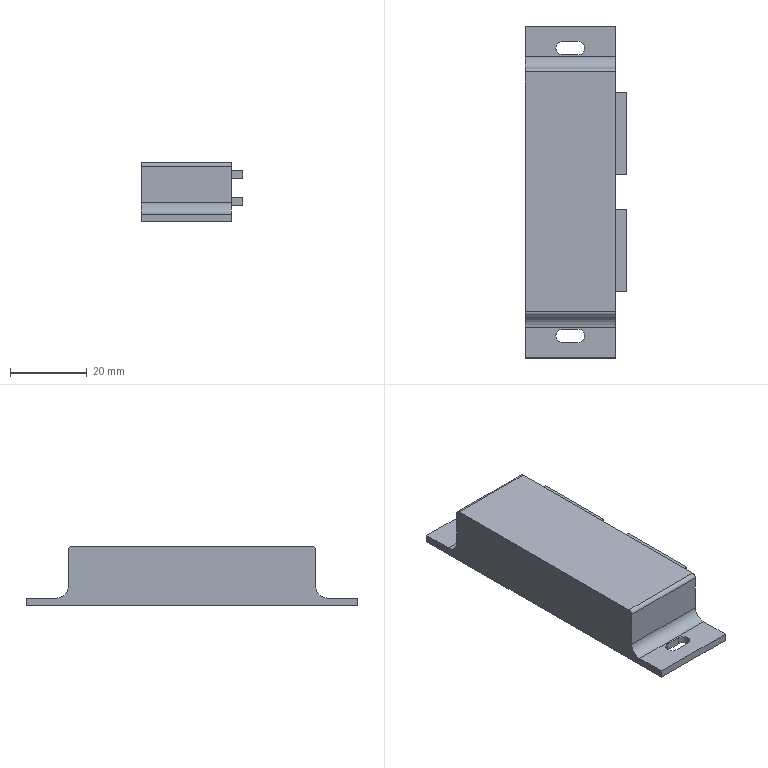Part | SolidWorks | features BaseBody 1 | 1 solid | 44 faces | box 26.5 x 86.5 x 15.5 mm | volume 25030 mm3 | plane 34 | cylinder 10 | commonest cylinder face diameters 3.5 x6 2 x2 6 x2
STEP:
#1=CARTESIAN_POINT('',(-2.,-35.75,2.));
#2=VERTEX_POINT('',#1);
#3=CARTESIAN_POINT('',(-3.75,-37.5,2.));
#4=VERTEX_POINT('',#3);
#5=CARTESIAN_POINT('',(-2.,-37.5,2.));
#6=DIRECTION('',(0.,0.,1.));
#7=DIRECTION('',(-1.,0.,0.));
#8=AXIS2_PLACEMENT_3D('',#5,#6,#7);
#9=CIRCLE('',#8,1.75);
#10=EDGE_CURVE('',#2,#4,#9,.T.);
#11=ORIENTED_EDGE('',*,*,#10,.T.);
#12=CARTESIAN_POINT('',(-3.75,-37.5,0.));
#13=VERTEX_POINT('',#12);
#14=CARTESIAN_POINT('',(-3.75,-37.5,3.));
#15=DIRECTION('',(0.,0.,-1.));
#16=VECTOR('',#15,1000.);
#17=LINE('',#14,#16);
#18=EDGE_CURVE('',#4,#13,#17,.T.);
#19=ORIENTED_EDGE('',*,*,#18,.T.);
#20=CARTESIAN_POINT('',(-2.,-35.75,0.));
#21=VERTEX_POINT('',#20);
#22=CARTESIAN_POINT('',(-2.,-37.5,0.));
#23=DIRECTION('',(0.,0.,1.));
#24=DIRECTION('',(1.,0.,0.));
#25=AXIS2_PLACEMENT_3D('',#22,#23,#24);
#26=CIRCLE('',#25,1.75);
#27=EDGE_CURVE('',#21,#13,#26,.T.);
#28=ORIENTED_EDGE('',*,*,#27,.F.);
#29=CARTESIAN_POINT('',(-2.,-35.75,3.));
#30=DIRECTION('',(0.,0.,-1.));
#31=VECTOR('',#30,1000.);
#32=LINE('',#29,#31);
#33=EDGE_CURVE('',#2,#21,#32,.T.);
#34=ORIENTED_EDGE('',*,*,#33,.F.);
#35=EDGE_LOOP('',(#11,#19,#28,#34));
#36=FACE_OUTER_BOUND('',#35,.T.);
#37=CARTESIAN_POINT('',(-2.,-37.5,3.));
#38=DIRECTION('',(0.,0.,-1.));
#39=DIRECTION('',(-1.,0.,0.));
#40=AXIS2_PLACEMENT_3D('',#37,#38,#39);
#41=CYLINDRICAL_SURFACE('',#40,1.75);
#42=ADVANCED_FACE('',(#36),#41,.F.);
#43=CARTESIAN_POINT('',(-2.,39.25,2.));
#44=VERTEX_POINT('',#43);
#45=CARTESIAN_POINT('',(-3.75,37.5,2.));
#46=VERTEX_POINT('',#45);
#47=CARTESIAN_POINT('',(-2.,37.5,2.));
#48=DIRECTION('',(0.,0.,1.));
#49=DIRECTION('',(-1.,0.,0.));
#50=AXIS2_PLACEMENT_3D('',#47,#48,#49);
#51=CIRCLE('',#50,1.75);
#52=EDGE_CURVE('',#44,#46,#51,.T.);
#53=ORIENTED_EDGE('',*,*,#52,.T.);
#54=CARTESIAN_POINT('',(-3.75,37.5,0.));
#55=VERTEX_POINT('',#54);
#56=CARTESIAN_POINT('',(-3.75,37.5,8.5));
#57=DIRECTION('',(0.,0.,-1.));
#58=VECTOR('',#57,1000.);
#59=LINE('',#56,#58);
#60=EDGE_CURVE('',#46,#55,#59,.T.);
#61=ORIENTED_EDGE('',*,*,#60,.T.);
#62=CARTESIAN_POINT('',(-2.,39.25,0.));
#63=VERTEX_POINT('',#62);
#64=CARTESIAN_POINT('',(-2.,37.5,0.));
#65=DIRECTION('',(0.,0.,-1.));
#66=DIRECTION('',(1.,0.,0.));
#67=AXIS2_PLACEMENT_3D('',#64,#65,#66);
#68=CIRCLE('',#67,1.75);
#69=EDGE_CURVE('',#55,#63,#68,.T.);
#70=ORIENTED_EDGE('',*,*,#69,.T.);
#71=CARTESIAN_POINT('',(-2.,39.25,8.5));
#72=DIRECTION('',(0.,0.,-1.));
#73=VECTOR('',#72,1000.);
#74=LINE('',#71,#73);
#75=EDGE_CURVE('',#44,#63,#74,.T.);
#76=ORIENTED_EDGE('',*,*,#75,.F.);
#77=EDGE_LOOP('',(#53,#61,#70,#76));
#78=FACE_OUTER_BOUND('',#77,.T.);
#79=CARTESIAN_POINT('',(-2.,37.5,8.5));
#80=DIRECTION('',(0.,0.,-1.));
#81=DIRECTION('',(-1.,0.,0.));
#82=AXIS2_PLACEMENT_3D('',#79,#80,#81);
#83=CYLINDRICAL_SURFACE('',#82,1.75);
#84=ADVANCED_FACE('',(#78),#83,.F.);
#85=CARTESIAN_POINT('',(14.75,-4.5,6.3));
#86=VERTEX_POINT('',#85);
#87=CARTESIAN_POINT('',(14.75,-4.5,4.3));
#88=VERTEX_POINT('',#87);
#89=CARTESIAN_POINT('',(14.75,-4.5,15.5));
#90=DIRECTION('',(0.,0.,-1.));
#91=VECTOR('',#90,1000.);
#92=LINE('',#89,#91);
#93=EDGE_CURVE('',#86,#88,#92,.T.);
#94=ORIENTED_EDGE('',*,*,#93,.T.);
#95=CARTESIAN_POINT('',(11.75,-4.5,4.3));
#96=VERTEX_POINT('',#95);
#97=CARTESIAN_POINT('',(14.75,-4.5,4.3));
#98=DIRECTION('',(1.,0.,0.));
#99=VECTOR('',#98,1000.);
#100=LINE('',#97,#99);
#101=EDGE_CURVE('',#96,#88,#100,.T.);
#102=ORIENTED_EDGE('',*,*,#101,.F.);
#103=CARTESIAN_POINT('',(11.75,-4.5,6.3));
#104=VERTEX_POINT('',#103);
#105=CARTESIAN_POINT('',(11.75,-4.5,15.5));
#106=DIRECTION('',(0.,0.,-1.));
#107=VECTOR('',#106,1000.);
#108=LINE('',#105,#107);
#109=EDGE_CURVE('',#104,#96,#108,.T.);
#110=ORIENTED_EDGE('',*,*,#109,.F.);
#111=CARTESIAN_POINT('',(14.75,-4.5,6.3));
#112=DIRECTION('',(-1.,0.,0.));
#113=VECTOR('',#112,1000.);
#114=LINE('',#111,#113);
#115=EDGE_CURVE('',#86,#104,#114,.T.);
#116=ORIENTED_EDGE('',*,*,#115,.F.);
#117=EDGE_LOOP('',(#94,#102,#110,#116));
#118=FACE_OUTER_BOUND('',#117,.T.);
#119=CARTESIAN_POINT('',(11.75,-4.5,15.5));
#120=DIRECTION('',(0.,-1.,0.));
#121=DIRECTION('',(0.,0.,-1.));
#122=AXIS2_PLACEMENT_3D('',#119,#120,#121);
#123=PLANE('',#122);
#124=ADVANCED_FACE('',(#118),#123,.F.);
#125=CARTESIAN_POINT('',(11.75,4.5,4.3));
#126=VERTEX_POINT('',#125);
#127=CARTESIAN_POINT('',(11.75,4.5,6.3));
#128=VERTEX_POINT('',#127);
#129=CARTESIAN_POINT('',(11.75,4.5,0.));
#130=DIRECTION('',(0.,0.,1.));
#131=VECTOR('',#130,1000.);
#132=LINE('',#129,#131);
#133=EDGE_CURVE('',#126,#128,#132,.T.);
#134=ORIENTED_EDGE('',*,*,#133,.F.);
#135=CARTESIAN_POINT('',(14.75,4.5,4.3));
#136=VERTEX_POINT('',#135);
#137=CARTESIAN_POINT('',(14.75,4.5,4.3));
#138=DIRECTION('',(-1.,0.,0.));
#139=VECTOR('',#138,1000.);
#140=LINE('',#137,#139);
#141=EDGE_CURVE('',#136,#126,#140,.T.);
#142=ORIENTED_EDGE('',*,*,#141,.F.);
#143=CARTESIAN_POINT('',(14.75,4.5,6.3));
#144=VERTEX_POINT('',#143);
#145=CARTESIAN_POINT('',(14.75,4.5,0.));
#146=DIRECTION('',(0.,0.,1.));
#147=VECTOR('',#146,1000.);
#148=LINE('',#145,#147);
#149=EDGE_CURVE('',#136,#144,#148,.T.);
#150=ORIENTED_EDGE('',*,*,#149,.T.);
#151=CARTESIAN_POINT('',(14.75,4.5,6.3));
#152=DIRECTION('',(1.,0.,0.));
#153=VECTOR('',#152,1000.);
#154=LINE('',#151,#153);
#155=EDGE_CURVE('',#128,#144,#154,.T.);
#156=ORIENTED_EDGE('',*,*,#155,.F.);
#157=EDGE_LOOP('',(#134,#142,#150,#156));
#158=FACE_OUTER_BOUND('',#157,.T.);
#159=CARTESIAN_POINT('',(11.75,4.5,0.));
#160=DIRECTION('',(0.,1.,0.));
#161=DIRECTION('',(1.,0.,0.));
#162=AXIS2_PLACEMENT_3D('',#159,#160,#161);
#163=PLANE('',#162);
#164=ADVANCED_FACE('',(#158),#163,.F.);
#165=CARTESIAN_POINT('',(11.75,4.5,11.3));
#166=VERTEX_POINT('',#165);
#167=CARTESIAN_POINT('',(11.75,4.5,13.3));
#168=VERTEX_POINT('',#167);
#169=CARTESIAN_POINT('',(11.75,4.5,0.));
#170=DIRECTION('',(0.,0.,1.));
#171=VECTOR('',#170,1000.);
#172=LINE('',#169,#171);
#173=EDGE_CURVE('',#166,#168,#172,.T.);
#174=ORIENTED_EDGE('',*,*,#173,.F.);
#175=CARTESIAN_POINT('',(14.75,4.5,11.3));
#176=VERTEX_POINT('',#175);
#177=CARTESIAN_POINT('',(14.75,4.5,11.3));
#178=DIRECTION('',(-1.,0.,0.));
#179=VECTOR('',#178,1000.);
#180=LINE('',#177,#179);
#181=EDGE_CURVE('',#176,#166,#180,.T.);
#182=ORIENTED_EDGE('',*,*,#181,.F.);
#183=CARTESIAN_POINT('',(14.75,4.5,13.3));
#184=VERTEX_POINT('',#183);
#185=CARTESIAN_POINT('',(14.75,4.5,0.));
#186=DIRECTION('',(0.,0.,1.));
#187=VECTOR('',#186,1000.);
#188=LINE('',#185,#187);
#189=EDGE_CURVE('',#176,#184,#188,.T.);
#190=ORIENTED_EDGE('',*,*,#189,.T.);
#191=CARTESIAN_POINT('',(14.75,4.5,13.3));
#192=DIRECTION('',(1.,0.,0.));
#193=VECTOR('',#192,1000.);
#194=LINE('',#191,#193);
#195=EDGE_CURVE('',#168,#184,#194,.T.);
#196=ORIENTED_EDGE('',*,*,#195,.F.);
#197=EDGE_LOOP('',(#174,#182,#190,#196));
#198=FACE_OUTER_BOUND('',#197,.T.);
#199=CARTESIAN_POINT('',(11.75,4.5,0.));
#200=DIRECTION('',(0.,1.,0.));
#201=DIRECTION('',(1.,0.,0.));
#202=AXIS2_PLACEMENT_3D('',#199,#200,#201);
#203=PLANE('',#202);
#204=ADVANCED_FACE('',(#198),#203,.F.);
#205=CARTESIAN_POINT('',(14.75,-4.5,13.3));
#206=VERTEX_POINT('',#205);
#207=CARTESIAN_POINT('',(14.75,-4.5,11.3));
#208=VERTEX_POINT('',#207);
#209=CARTESIAN_POINT('',(14.75,-4.5,0.));
#210=DIRECTION('',(0.,0.,-1.));
#211=VECTOR('',#210,1000.);
#212=LINE('',#209,#211);
#213=EDGE_CURVE('',#206,#208,#212,.T.);
#214=ORIENTED_EDGE('',*,*,#213,.T.);
#215=CARTESIAN_POINT('',(11.75,-4.5,11.3));
#216=VERTEX_POINT('',#215);
#217=CARTESIAN_POINT('',(14.75,-4.5,11.3));
#218=DIRECTION('',(1.,0.,0.));
#219=VECTOR('',#218,1000.);
#220=LINE('',#217,#219);
#221=EDGE_CURVE('',#216,#208,#220,.T.);
#222=ORIENTED_EDGE('',*,*,#221,.F.);
#223=CARTESIAN_POINT('',(11.75,-4.5,13.3));
#224=VERTEX_POINT('',#223);
#225=CARTESIAN_POINT('',(11.75,-4.5,15.5));
#226=DIRECTION('',(0.,0.,-1.));
#227=VECTOR('',#226,1000.);
#228=LINE('',#225,#227);
#229=EDGE_CURVE('',#224,#216,#228,.T.);
#230=ORIENTED_EDGE('',*,*,#229,.F.);
#231=CARTESIAN_POINT('',(14.75,-4.5,13.3));
#232=DIRECTION('',(-1.,0.,0.));
#233=VECTOR('',#232,1000.);
#234=LINE('',#231,#233);
#235=EDGE_CURVE('',#206,#224,#234,.T.);
#236=ORIENTED_EDGE('',*,*,#235,.F.);
#237=EDGE_LOOP('',(#214,#222,#230,#236));
#238=FACE_OUTER_BOUND('',#237,.T.);
#239=CARTESIAN_POINT('',(11.75,-4.5,15.5));
#240=DIRECTION('',(0.,-1.,0.));
#241=DIRECTION('',(0.,0.,-1.));
#242=AXIS2_PLACEMENT_3D('',#239,#240,#241);
#243=PLANE('',#242);
#244=ADVANCED_FACE('',(#238),#243,.F.);
#245=CARTESIAN_POINT('',(2.,-35.75,2.));
#246=VERTEX_POINT('',#245);
#247=CARTESIAN_POINT('',(11.75,-35.75,2.));
#248=DIRECTION('',(-1.,0.,0.));
#249=VECTOR('',#248,1000.);
#250=LINE('',#247,#249);
#251=EDGE_CURVE('',#246,#2,#250,.T.);
#252=ORIENTED_EDGE('',*,*,#251,.T.);
#253=ORIENTED_EDGE('',*,*,#33,.T.);
#254=CARTESIAN_POINT('',(2.,-35.75,0.));
#255=VERTEX_POINT('',#254);
#256=CARTESIAN_POINT('',(2.,-35.75,0.));
#257=DIRECTION('',(-1.,0.,0.));
#258=VECTOR('',#257,1000.);
#259=LINE('',#256,#258);
#260=EDGE_CURVE('',#255,#21,#259,.T.);
#261=ORIENTED_EDGE('',*,*,#260,.F.);
#262=CARTESIAN_POINT('',(2.,-35.75,3.));
#263=DIRECTION('',(0.,0.,-1.));
#264=VECTOR('',#263,1000.);
#265=LINE('',#262,#264);
#266=EDGE_CURVE('',#246,#255,#265,.T.);
#267=ORIENTED_EDGE('',*,*,#266,.F.);
#268=EDGE_LOOP('',(#252,#253,#261,#267));
#269=FACE_OUTER_BOUND('',#268,.T.);
#270=CARTESIAN_POINT('',(2.,-35.75,3.));
#271=DIRECTION('',(0.,-1.,0.));
#272=DIRECTION('',(0.,0.,-1.));
#273=AXIS2_PLACEMENT_3D('',#270,#271,#272);
#274=PLANE('',#273);
#275=ADVANCED_FACE('',(#269),#274,.T.);
#276=CARTESIAN_POINT('',(2.,-39.25,2.));
#277=VERTEX_POINT('',#276);
#278=CARTESIAN_POINT('',(2.,-37.5,2.));
#279=DIRECTION('',(0.,0.,1.));
#280=DIRECTION('',(-1.,0.,0.));
#281=AXIS2_PLACEMENT_3D('',#278,#279,#280);
#282=CIRCLE('',#281,1.75);
#283=EDGE_CURVE('',#277,#246,#282,.T.);
#284=ORIENTED_EDGE('',*,*,#283,.T.);
#285=ORIENTED_EDGE('',*,*,#266,.T.);
#286=CARTESIAN_POINT('',(2.,-39.25,0.));
#287=VERTEX_POINT('',#286);
#288=CARTESIAN_POINT('',(2.,-37.5,0.));
#289=DIRECTION('',(0.,0.,1.));
#290=DIRECTION('',(1.,0.,0.));
#291=AXIS2_PLACEMENT_3D('',#288,#289,#290);
#292=CIRCLE('',#291,1.75);
#293=EDGE_CURVE('',#287,#255,#292,.T.);
#294=ORIENTED_EDGE('',*,*,#293,.F.);
#295=CARTESIAN_POINT('',(2.,-39.25,3.));
#296=DIRECTION('',(0.,0.,-1.));
#297=VECTOR('',#296,1000.);
#298=LINE('',#295,#297);
#299=EDGE_CURVE('',#277,#287,#298,.T.);
#300=ORIENTED_EDGE('',*,*,#299,.F.);
#301=EDGE_LOOP('',(#284,#285,#294,#300));
#302=FACE_OUTER_BOUND('',#301,.T.);
#303=CARTESIAN_POINT('',(2.,-37.5,3.));
#304=DIRECTION('',(0.,0.,-1.));
#305=DIRECTION('',(-1.,0.,0.));
#306=AXIS2_PLACEMENT_3D('',#303,#304,#305);
#307=CYLINDRICAL_SURFACE('',#306,1.75);
#308=ADVANCED_FACE('',(#302),#307,.F.);
#309=CARTESIAN_POINT('',(-2.,-39.25,2.));
#310=VERTEX_POINT('',#309);
#311=CARTESIAN_POINT('',(11.75,-39.25,2.));
#312=DIRECTION('',(1.,0.,0.));
#313=VECTOR('',#312,1000.);
#314=LINE('',#311,#313);
#315=EDGE_CURVE('',#310,#277,#314,.T.);
#316=ORIENTED_EDGE('',*,*,#315,.T.);
#317=ORIENTED_EDGE('',*,*,#299,.T.);
#318=CARTESIAN_POINT('',(-2.,-39.25,0.));
#319=VERTEX_POINT('',#318);
#320=CARTESIAN_POINT('',(-2.,-39.25,0.));
#321=DIRECTION('',(1.,0.,0.));
#322=VECTOR('',#321,1000.);
#323=LINE('',#320,#322);
#324=EDGE_CURVE('',#319,#287,#323,.T.);
#325=ORIENTED_EDGE('',*,*,#324,.F.);
#326=CARTESIAN_POINT('',(-2.,-39.25,3.));
#327=DIRECTION('',(0.,0.,-1.));
#328=VECTOR('',#327,1000.);
#329=LINE('',#326,#328);
#330=EDGE_CURVE('',#310,#319,#329,.T.);
#331=ORIENTED_EDGE('',*,*,#330,.F.);
#332=EDGE_LOOP('',(#316,#317,#325,#331));
#333=FACE_OUTER_BOUND('',#332,.T.);
#334=CARTESIAN_POINT('',(-2.,-39.25,3.));
#335=DIRECTION('',(0.,1.,0.));
#336=DIRECTION('',(1.,0.,0.));
#337=AXIS2_PLACEMENT_3D('',#334,#335,#336);
#338=PLANE('',#337);
#339=ADVANCED_FACE('',(#333),#338,.T.);
#340=ORIENTED_EDGE('',*,*,#213,.F.);
#341=CARTESIAN_POINT('',(14.75,-26.,13.3));
#342=VERTEX_POINT('',#341);
#343=CARTESIAN_POINT('',(14.75,26.,13.3));
#344=DIRECTION('',(0.,-1.,0.));
#345=VECTOR('',#344,1000.);
#346=LINE('',#343,#345);
#347=EDGE_CURVE('',#206,#342,#346,.T.);
#348=ORIENTED_EDGE('',*,*,#347,.T.);
#349=CARTESIAN_POINT('',(14.75,-26.,11.3));
#350=VERTEX_POINT('',#349);
#351=CARTESIAN_POINT('',(14.75,-26.,13.3));
#352=DIRECTION('',(0.,0.,-1.));
#353=VECTOR('',#352,1000.);
#354=LINE('',#351,#353);
#355=EDGE_CURVE('',#342,#350,#354,.T.);
#356=ORIENTED_EDGE('',*,*,#355,.T.);
#357=CARTESIAN_POINT('',(14.75,-26.,11.3));
#358=DIRECTION('',(0.,1.,0.));
#359=VECTOR('',#358,1000.);
#360=LINE('',#357,#359);
#361=EDGE_CURVE('',#350,#208,#360,.T.);
#362=ORIENTED_EDGE('',*,*,#361,.T.);
#363=EDGE_LOOP('',(#340,#348,#356,#362));
#364=FACE_OUTER_BOUND('',#363,.T.);
#365=CARTESIAN_POINT('',(14.75,0.,0.));
#366=DIRECTION('',(1.,0.,0.));
#367=DIRECTION('',(0.,1.,0.));
#368=AXIS2_PLACEMENT_3D('',#365,#366,#367);
#369=PLANE('',#368);
#370=ADVANCED_FACE('',(#364),#369,.T.);
#371=CARTESIAN_POINT('',(11.75,-26.,11.3));
#372=VERTEX_POINT('',#371);
#373=CARTESIAN_POINT('',(11.75,31.25,11.3));
#374=DIRECTION('',(0.,-1.,0.));
#375=VECTOR('',#374,1000.);
#376=LINE('',#373,#375);
#377=EDGE_CURVE('',#216,#372,#376,.T.);
#378=ORIENTED_EDGE('',*,*,#377,.F.);
#379=ORIENTED_EDGE('',*,*,#221,.T.);
#380=ORIENTED_EDGE('',*,*,#361,.F.);
#381=CARTESIAN_POINT('',(14.75,-26.,11.3));
#382=DIRECTION('',(-1.,0.,0.));
#383=VECTOR('',#382,1000.);
#384=LINE('',#381,#383);
#385=EDGE_CURVE('',#350,#372,#384,.T.);
#386=ORIENTED_EDGE('',*,*,#385,.T.);
#387=EDGE_LOOP('',(#378,#379,#380,#386));
#388=FACE_OUTER_BOUND('',#387,.T.);
#389=CARTESIAN_POINT('',(14.75,-26.,11.3));
#390=DIRECTION('',(0.,0.,1.));
#391=DIRECTION('',(1.,0.,0.));
#392=AXIS2_PLACEMENT_3D('',#389,#390,#391);
#393=PLANE('',#392);
#394=ADVANCED_FACE('',(#388),#393,.F.);
#395=CARTESIAN_POINT('',(11.75,-26.,13.3));
#396=VERTEX_POINT('',#395);
#397=CARTESIAN_POINT('',(11.75,-26.,14.5));
#398=DIRECTION('',(0.,0.,1.));
#399=VECTOR('',#398,1000.);
#400=LINE('',#397,#399);
#401=EDGE_CURVE('',#372,#396,#400,.T.);
#402=ORIENTED_EDGE('',*,*,#401,.F.);
#403=ORIENTED_EDGE('',*,*,#385,.F.);
#404=ORIENTED_EDGE('',*,*,#355,.F.);
#405=CARTESIAN_POINT('',(14.75,-26.,13.3));
#406=DIRECTION('',(-1.,0.,0.));
#407=VECTOR('',#406,1000.);
#408=LINE('',#405,#407);
#409=EDGE_CURVE('',#342,#396,#408,.T.);
#410=ORIENTED_EDGE('',*,*,#409,.T.);
#411=EDGE_LOOP('',(#402,#403,#404,#410));
#412=FACE_OUTER_BOUND('',#411,.T.);
#413=CARTESIAN_POINT('',(14.75,-26.,13.3));
#414=DIRECTION('',(0.,1.,0.));
#415=DIRECTION('',(1.,0.,0.));
#416=AXIS2_PLACEMENT_3D('',#413,#414,#415);
#417=PLANE('',#416);
#418=ADVANCED_FACE('',(#412),#417,.F.);
#419=ORIENTED_EDGE('',*,*,#347,.F.);
#420=ORIENTED_EDGE('',*,*,#235,.T.);
#421=CARTESIAN_POINT('',(11.75,31.25,13.3));
#422=DIRECTION('',(0.,1.,0.));
#423=VECTOR('',#422,1000.);
#424=LINE('',#421,#423);
#425=EDGE_CURVE('',#396,#224,#424,.T.);
#426=ORIENTED_EDGE('',*,*,#425,.F.);
#427=ORIENTED_EDGE('',*,*,#409,.F.);
#428=EDGE_LOOP('',(#419,#420,#426,#427));
#429=FACE_OUTER_BOUND('',#428,.T.);
#430=CARTESIAN_POINT('',(14.75,26.,13.3));
#431=DIRECTION('',(0.,0.,-1.));
#432=DIRECTION('',(0.,-1.,0.));
#433=AXIS2_PLACEMENT_3D('',#430,#431,#432);
#434=PLANE('',#433);
#435=ADVANCED_FACE('',(#429),#434,.F.);
#436=CARTESIAN_POINT('',(11.75,26.,13.3));
#437=VERTEX_POINT('',#436);
#438=CARTESIAN_POINT('',(11.75,26.,11.3));
#439=VERTEX_POINT('',#438);
#440=CARTESIAN_POINT('',(11.75,26.,14.5));
#441=DIRECTION('',(0.,0.,-1.));
#442=VECTOR('',#441,1000.);
#443=LINE('',#440,#442);
#444=EDGE_CURVE('',#437,#439,#443,.T.);
#445=ORIENTED_EDGE('',*,*,#444,.F.);
#446=CARTESIAN_POINT('',(14.75,26.,13.3));
#447=VERTEX_POINT('',#446);
#448=CARTESIAN_POINT('',(14.75,26.,13.3));
#449=DIRECTION('',(-1.,0.,0.));
#450=VECTOR('',#449,1000.);
#451=LINE('',#448,#450);
#452=EDGE_CURVE('',#447,#437,#451,.T.);
#453=ORIENTED_EDGE('',*,*,#452,.F.);
#454=CARTESIAN_POINT('',(14.75,26.,11.3));
#455=VERTEX_POINT('',#454);
#456=CARTESIAN_POINT('',(14.75,26.,11.3));
#457=DIRECTION('',(0.,0.,1.));
#458=VECTOR('',#457,1000.);
#459=LINE('',#456,#458);
#460=EDGE_CURVE('',#455,#447,#459,.T.);
#461=ORIENTED_EDGE('',*,*,#460,.F.);
#462=CARTESIAN_POINT('',(14.75,26.,11.3));
#463=DIRECTION('',(-1.,0.,0.));
#464=VECTOR('',#463,1000.);
#465=LINE('',#462,#464);
#466=EDGE_CURVE('',#455,#439,#465,.T.);
#467=ORIENTED_EDGE('',*,*,#466,.T.);
#468=EDGE_LOOP('',(#445,#453,#461,#467));
#469=FACE_OUTER_BOUND('',#468,.T.);
#470=CARTESIAN_POINT('',(14.75,26.,11.3));
#471=DIRECTION('',(0.,-1.,0.));
#472=DIRECTION('',(0.,0.,-1.));
#473=AXIS2_PLACEMENT_3D('',#470,#471,#472);
#474=PLANE('',#473);
#475=ADVANCED_FACE('',(#469),#474,.F.);
#476=ORIENTED_EDGE('',*,*,#93,.F.);
#477=CARTESIAN_POINT('',(14.75,-26.,6.3));
#478=VERTEX_POINT('',#477);
#479=CARTESIAN_POINT('',(14.75,26.,6.3));
#480=DIRECTION('',(0.,-1.,0.));
#481=VECTOR('',#480,1000.);
#482=LINE('',#479,#481);
#483=EDGE_CURVE('',#86,#478,#482,.T.);
#484=ORIENTED_EDGE('',*,*,#483,.T.);
#485=CARTESIAN_POINT('',(14.75,-26.,4.3));
#486=VERTEX_POINT('',#485);
#487=CARTESIAN_POINT('',(14.75,-26.,6.3));
#488=DIRECTION('',(0.,0.,-1.));
#489=VECTOR('',#488,1000.);
#490=LINE('',#487,#489);
#491=EDGE_CURVE('',#478,#486,#490,.T.);
#492=ORIENTED_EDGE('',*,*,#491,.T.);
#493=CARTESIAN_POINT('',(14.75,-26.,4.3));
#494=DIRECTION('',(0.,1.,0.));
#495=VECTOR('',#494,1000.);
#496=LINE('',#493,#495);
#497=EDGE_CURVE('',#486,#88,#496,.T.);
#498=ORIENTED_EDGE('',*,*,#497,.T.);
#499=EDGE_LOOP('',(#476,#484,#492,#498));
#500=FACE_OUTER_BOUND('',#499,.T.);
#501=CARTESIAN_POINT('',(14.75,0.,0.));
#502=DIRECTION('',(1.,0.,0.));
#503=DIRECTION('',(0.,1.,0.));
#504=AXIS2_PLACEMENT_3D('',#501,#502,#503);
#505=PLANE('',#504);
#506=ADVANCED_FACE('',(#500),#505,.T.);
#507=CARTESIAN_POINT('',(11.75,-26.,4.3));
#508=VERTEX_POINT('',#507);
#509=CARTESIAN_POINT('',(11.75,31.25,4.3));
#510=DIRECTION('',(0.,-1.,0.));
#511=VECTOR('',#510,1000.);
#512=LINE('',#509,#511);
#513=EDGE_CURVE('',#96,#508,#512,.T.);
#514=ORIENTED_EDGE('',*,*,#513,.F.);
#515=ORIENTED_EDGE('',*,*,#101,.T.);
#516=ORIENTED_EDGE('',*,*,#497,.F.);
#517=CARTESIAN_POINT('',(14.75,-26.,4.3));
#518=DIRECTION('',(-1.,0.,0.));
#519=VECTOR('',#518,1000.);
#520=LINE('',#517,#519);
#521=EDGE_CURVE('',#486,#508,#520,.T.);
#522=ORIENTED_EDGE('',*,*,#521,.T.);
#523=EDGE_LOOP('',(#514,#515,#516,#522));
#524=FACE_OUTER_BOUND('',#523,.T.);
#525=CARTESIAN_POINT('',(14.75,-26.,4.3));
#526=DIRECTION('',(0.,0.,1.));
#527=DIRECTION('',(1.,0.,0.));
#528=AXIS2_PLACEMENT_3D('',#525,#526,#527);
#529=PLANE('',#528);
#530=ADVANCED_FACE('',(#524),#529,.F.);
#531=CARTESIAN_POINT('',(11.75,-26.,6.3));
#532=VERTEX_POINT('',#531);
#533=CARTESIAN_POINT('',(11.75,-26.,14.5));
#534=DIRECTION('',(0.,0.,1.));
#535=VECTOR('',#534,1000.);
#536=LINE('',#533,#535);
#537=EDGE_CURVE('',#508,#532,#536,.T.);
#538=ORIENTED_EDGE('',*,*,#537,.F.);
#539=ORIENTED_EDGE('',*,*,#521,.F.);
#540=ORIENTED_EDGE('',*,*,#491,.F.);
#541=CARTESIAN_POINT('',(14.75,-26.,6.3));
#542=DIRECTION('',(-1.,0.,0.));
#543=VECTOR('',#542,1000.);
#544=LINE('',#541,#543);
#545=EDGE_CURVE('',#478,#532,#544,.T.);
#546=ORIENTED_EDGE('',*,*,#545,.T.);
#547=EDGE_LOOP('',(#538,#539,#540,#546));
#548=FACE_OUTER_BOUND('',#547,.T.);
#549=CARTESIAN_POINT('',(14.75,-26.,6.3));
#550=DIRECTION('',(0.,1.,0.));
#551=DIRECTION('',(1.,0.,0.));
#552=AXIS2_PLACEMENT_3D('',#549,#550,#551);
#553=PLANE('',#552);
#554=ADVANCED_FACE('',(#548),#553,.F.);
#555=ORIENTED_EDGE('',*,*,#483,.F.);
#556=ORIENTED_EDGE('',*,*,#115,.T.);
#557=CARTESIAN_POINT('',(11.75,31.25,6.3));
#558=DIRECTION('',(0.,1.,0.));
#559=VECTOR('',#558,1000.);
#560=LINE('',#557,#559);
#561=EDGE_CURVE('',#532,#104,#560,.T.);
#562=ORIENTED_EDGE('',*,*,#561,.F.);
#563=ORIENTED_EDGE('',*,*,#545,.F.);
#564=EDGE_LOOP('',(#555,#556,#562,#563));
#565=FACE_OUTER_BOUND('',#564,.T.);
#566=CARTESIAN_POINT('',(14.75,26.,6.3));
#567=DIRECTION('',(0.,0.,-1.));
#568=DIRECTION('',(0.,-1.,0.));
#569=AXIS2_PLACEMENT_3D('',#566,#567,#568);
#570=PLANE('',#569);
#571=ADVANCED_FACE('',(#565),#570,.F.);
#572=CARTESIAN_POINT('',(11.75,26.,6.3));
#573=VERTEX_POINT('',#572);
#574=CARTESIAN_POINT('',(11.75,26.,4.3));
#575=VERTEX_POINT('',#574);
#576=CARTESIAN_POINT('',(11.75,26.,14.5));
#577=DIRECTION('',(0.,0.,-1.));
#578=VECTOR('',#577,1000.);
#579=LINE('',#576,#578);
#580=EDGE_CURVE('',#573,#575,#579,.T.);
#581=ORIENTED_EDGE('',*,*,#580,.F.);
#582=CARTESIAN_POINT('',(14.75,26.,6.3));
#583=VERTEX_POINT('',#582);
#584=CARTESIAN_POINT('',(14.75,26.,6.3));
#585=DIRECTION('',(-1.,0.,0.));
#586=VECTOR('',#585,1000.);
#587=LINE('',#584,#586);
#588=EDGE_CURVE('',#583,#573,#587,.T.);
#589=ORIENTED_EDGE('',*,*,#588,.F.);
#590=CARTESIAN_POINT('',(14.75,26.,4.3));
#591=VERTEX_POINT('',#590);
#592=CARTESIAN_POINT('',(14.75,26.,4.3));
#593=DIRECTION('',(0.,0.,1.));
#594=VECTOR('',#593,1000.);
#595=LINE('',#592,#594);
#596=EDGE_CURVE('',#591,#583,#595,.T.);
#597=ORIENTED_EDGE('',*,*,#596,.F.);
#598=CARTESIAN_POINT('',(14.75,26.,4.3));
#599=DIRECTION('',(-1.,0.,0.));
#600=VECTOR('',#599,1000.);
#601=LINE('',#598,#600);
#602=EDGE_CURVE('',#591,#575,#601,.T.);
#603=ORIENTED_EDGE('',*,*,#602,.T.);
#604=EDGE_LOOP('',(#581,#589,#597,#603));
#605=FACE_OUTER_BOUND('',#604,.T.);
#606=CARTESIAN_POINT('',(14.75,26.,4.3));
#607=DIRECTION('',(0.,-1.,0.));
#608=DIRECTION('',(0.,0.,-1.));
#609=AXIS2_PLACEMENT_3D('',#606,#607,#608);
#610=PLANE('',#609);
#611=ADVANCED_FACE('',(#605),#610,.F.);
#612=CARTESIAN_POINT('',(2.,39.25,0.));
#613=VERTEX_POINT('',#612);
#614=CARTESIAN_POINT('',(11.75,39.25,0.));
#615=DIRECTION('',(1.,0.,0.));
#616=VECTOR('',#615,1000.);
#617=LINE('',#614,#616);
#618=EDGE_CURVE('',#63,#613,#617,.T.);
#619=ORIENTED_EDGE('',*,*,#618,.T.);
#620=CARTESIAN_POINT('',(2.,39.25,2.));
#621=VERTEX_POINT('',#620);
#622=CARTESIAN_POINT('',(2.,39.25,8.5));
#623=DIRECTION('',(0.,0.,-1.));
#624=VECTOR('',#623,1000.);
#625=LINE('',#622,#624);
#626=EDGE_CURVE('',#621,#613,#625,.T.);
#627=ORIENTED_EDGE('',*,*,#626,.F.);
#628=CARTESIAN_POINT('',(11.75,39.25,2.));
#629=DIRECTION('',(-1.,0.,0.));
#630=VECTOR('',#629,1000.);
#631=LINE('',#628,#630);
#632=EDGE_CURVE('',#621,#44,#631,.T.);
#633=ORIENTED_EDGE('',*,*,#632,.T.);
#634=ORIENTED_EDGE('',*,*,#75,.T.);
#635=EDGE_LOOP('',(#619,#627,#633,#634));
#636=FACE_OUTER_BOUND('',#635,.T.);
#637=CARTESIAN_POINT('',(2.,39.25,8.5));
#638=DIRECTION('',(0.,-1.,0.));
#639=DIRECTION('',(0.,0.,-1.));
#640=AXIS2_PLACEMENT_3D('',#637,#638,#639);
#641=PLANE('',#640);
#642=ADVANCED_FACE('',(#636),#641,.T.);
#643=CARTESIAN_POINT('',(2.,35.75,0.));
#644=VERTEX_POINT('',#643);
#645=CARTESIAN_POINT('',(2.,37.5,0.));
#646=DIRECTION('',(0.,0.,-1.));
#647=DIRECTION('',(1.,0.,0.));
#648=AXIS2_PLACEMENT_3D('',#645,#646,#647);
#649=CIRCLE('',#648,1.75);
#650=EDGE_CURVE('',#613,#644,#649,.T.);
#651=ORIENTED_EDGE('',*,*,#650,.T.);
#652=CARTESIAN_POINT('',(2.,35.75,2.));
#653=VERTEX_POINT('',#652);
#654=CARTESIAN_POINT('',(2.,35.75,8.5));
#655=DIRECTION('',(0.,0.,-1.));
#656=VECTOR('',#655,1000.);
#657=LINE('',#654,#656);
#658=EDGE_CURVE('',#653,#644,#657,.T.);
#659=ORIENTED_EDGE('',*,*,#658,.F.);
#660=CARTESIAN_POINT('',(2.,37.5,2.));
#661=DIRECTION('',(0.,0.,1.));
#662=DIRECTION('',(-1.,0.,0.));
#663=AXIS2_PLACEMENT_3D('',#660,#661,#662);
#664=CIRCLE('',#663,1.75);
#665=EDGE_CURVE('',#653,#621,#664,.T.);
#666=ORIENTED_EDGE('',*,*,#665,.T.);
#667=ORIENTED_EDGE('',*,*,#626,.T.);
#668=EDGE_LOOP('',(#651,#659,#666,#667));
#669=FACE_OUTER_BOUND('',#668,.T.);
#670=CARTESIAN_POINT('',(2.,37.5,8.5));
#671=DIRECTION('',(0.,0.,-1.));
#672=DIRECTION('',(-1.,0.,0.));
#673=AXIS2_PLACEMENT_3D('',#670,#671,#672);
#674=CYLINDRICAL_SURFACE('',#673,1.75);
#675=ADVANCED_FACE('',(#669),#674,.F.);
#676=CARTESIAN_POINT('',(-2.,35.75,0.));
#677=VERTEX_POINT('',#676);
#678=CARTESIAN_POINT('',(11.75,35.75,0.));
#679=DIRECTION('',(-1.,0.,0.));
#680=VECTOR('',#679,1000.);
#681=LINE('',#678,#680);
#682=EDGE_CURVE('',#644,#677,#681,.T.);
#683=ORIENTED_EDGE('',*,*,#682,.T.);
#684=CARTESIAN_POINT('',(-2.,35.75,2.));
#685=VERTEX_POINT('',#684);
#686=CARTESIAN_POINT('',(-2.,35.75,8.5));
#687=DIRECTION('',(0.,0.,-1.));
#688=VECTOR('',#687,1000.);
#689=LINE('',#686,#688);
#690=EDGE_CURVE('',#685,#677,#689,.T.);
#691=ORIENTED_EDGE('',*,*,#690,.F.);
#692=CARTESIAN_POINT('',(11.75,35.75,2.));
#693=DIRECTION('',(1.,0.,0.));
#694=VECTOR('',#693,1000.);
#695=LINE('',#692,#694);
#696=EDGE_CURVE('',#685,#653,#695,.T.);
#697=ORIENTED_EDGE('',*,*,#696,.T.);
#698=ORIENTED_EDGE('',*,*,#658,.T.);
#699=EDGE_LOOP('',(#683,#691,#697,#698));
#700=FACE_OUTER_BOUND('',#699,.T.);
#701=CARTESIAN_POINT('',(-2.,35.75,8.5));
#702=DIRECTION('',(0.,1.,0.));
#703=DIRECTION('',(1.,0.,0.));
#704=AXIS2_PLACEMENT_3D('',#701,#702,#703);
#705=PLANE('',#704);
#706=ADVANCED_FACE('',(#700),#705,.T.);
#707=CARTESIAN_POINT('',(-11.75,32.25,14.5));
#708=VERTEX_POINT('',#707);
#709=CARTESIAN_POINT('',(-11.75,31.25,15.5));
#710=VERTEX_POINT('',#709);
#711=CARTESIAN_POINT('',(-11.75,31.25,14.5));
#712=DIRECTION('',(1.,0.,0.));
#713=DIRECTION('',(0.,0.,-1.));
#714=AXIS2_PLACEMENT_3D('',#711,#712,#713);
#715=CIRCLE('',#714,1.);
#716=EDGE_CURVE('',#708,#710,#715,.T.);
#717=ORIENTED_EDGE('',*,*,#716,.F.);
#718=CARTESIAN_POINT('',(-11.75,32.25,5.));
#719=VERTEX_POINT('',#718);
#720=CARTESIAN_POINT('',(-11.75,32.25,5.));
#721=DIRECTION('',(0.,0.,1.));
#722=VECTOR('',#721,1000.);
#723=LINE('',#720,#722);
#724=EDGE_CURVE('',#719,#708,#723,.T.);
#725=ORIENTED_EDGE('',*,*,#724,.F.);
#726=CARTESIAN_POINT('',(-11.75,35.25,2.));
#727=VERTEX_POINT('',#726);
#728=CARTESIAN_POINT('',(-11.75,35.25,5.));
#729=DIRECTION('',(-1.,0.,0.));
#730=DIRECTION('',(0.,0.,1.));
#731=AXIS2_PLACEMENT_3D('',#728,#729,#730);
#732=CIRCLE('',#731,3.);
#733=EDGE_CURVE('',#727,#719,#732,.T.);
#734=ORIENTED_EDGE('',*,*,#733,.F.);
#735=CARTESIAN_POINT('',(-11.75,43.25,2.));
#736=VERTEX_POINT('',#735);
#737=CARTESIAN_POINT('',(-11.75,43.25,2.));
#738=DIRECTION('',(0.,-1.,0.));
#739=VECTOR('',#738,1000.);
#740=LINE('',#737,#739);
#741=EDGE_CURVE('',#736,#727,#740,.T.);
#742=ORIENTED_EDGE('',*,*,#741,.F.);
#743=CARTESIAN_POINT('',(-11.75,43.25,0.));
#744=VERTEX_POINT('',#743);
#745=CARTESIAN_POINT('',(-11.75,43.25,0.));
#746=DIRECTION('',(0.,0.,1.));
#747=VECTOR('',#746,1000.);
#748=LINE('',#745,#747);
#749=EDGE_CURVE('',#744,#736,#748,.T.);
#750=ORIENTED_EDGE('',*,*,#749,.F.);
#751=CARTESIAN_POINT('',(-11.75,-43.25,0.));
#752=VERTEX_POINT('',#751);
#753=CARTESIAN_POINT('',(-11.75,-43.25,0.));
#754=DIRECTION('',(0.,1.,0.));
#755=VECTOR('',#754,1000.);
#756=LINE('',#753,#755);
#757=EDGE_CURVE('',#752,#744,#756,.T.);
#758=ORIENTED_EDGE('',*,*,#757,.F.);
#759=CARTESIAN_POINT('',(-11.75,-43.25,2.));
#760=VERTEX_POINT('',#759);
#761=CARTESIAN_POINT('',(-11.75,-43.25,2.));
#762=DIRECTION('',(0.,0.,-1.));
#763=VECTOR('',#762,1000.);
#764=LINE('',#761,#763);
#765=EDGE_CURVE('',#760,#752,#764,.T.);
#766=ORIENTED_EDGE('',*,*,#765,.F.);
#767=CARTESIAN_POINT('',(-11.75,-35.25,2.));
#768=VERTEX_POINT('',#767);
#769=CARTESIAN_POINT('',(-11.75,-35.25,2.));
#770=DIRECTION('',(0.,-1.,0.));
#771=VECTOR('',#770,1000.);
#772=LINE('',#769,#771);
#773=EDGE_CURVE('',#768,#760,#772,.T.);
#774=ORIENTED_EDGE('',*,*,#773,.F.);
#775=CARTESIAN_POINT('',(-11.75,-32.25,5.));
#776=VERTEX_POINT('',#775);
#777=CARTESIAN_POINT('',(-11.75,-35.25,5.));
#778=DIRECTION('',(-1.,0.,0.));
#779=DIRECTION('',(0.,0.,1.));
#780=AXIS2_PLACEMENT_3D('',#777,#778,#779);
#781=CIRCLE('',#780,3.);
#782=EDGE_CURVE('',#776,#768,#781,.T.);
#783=ORIENTED_EDGE('',*,*,#782,.F.);
#784=CARTESIAN_POINT('',(-11.75,-32.25,14.5));
#785=VERTEX_POINT('',#784);
#786=CARTESIAN_POINT('',(-11.75,-32.25,14.5));
#787=DIRECTION('',(0.,0.,-1.));
#788=VECTOR('',#787,1000.);
#789=LINE('',#786,#788);
#790=EDGE_CURVE('',#785,#776,#789,.T.);
#791=ORIENTED_EDGE('',*,*,#790,.F.);
#792=CARTESIAN_POINT('',(-11.75,-31.25,15.5));
#793=VERTEX_POINT('',#792);
#794=CARTESIAN_POINT('',(-11.75,-31.25,14.5));
#795=DIRECTION('',(1.,0.,0.));
#796=DIRECTION('',(0.,0.,-1.));
#797=AXIS2_PLACEMENT_3D('',#794,#795,#796);
#798=CIRCLE('',#797,1.);
#799=EDGE_CURVE('',#793,#785,#798,.T.);
#800=ORIENTED_EDGE('',*,*,#799,.F.);
#801=CARTESIAN_POINT('',(-11.75,31.25,15.5));
#802=DIRECTION('',(0.,-1.,0.));
#803=VECTOR('',#802,1000.);
#804=LINE('',#801,#803);
#805=EDGE_CURVE('',#710,#793,#804,.T.);
#806=ORIENTED_EDGE('',*,*,#805,.F.);
#807=EDGE_LOOP('',(#717,#725,#734,#742,#750,#758,#766,#774,#783,#791,#800,#806));
#808=FACE_OUTER_BOUND('',#807,.T.);
#809=CARTESIAN_POINT('',(-11.75,31.25,14.5));
#810=DIRECTION('',(1.,0.,0.));
#811=DIRECTION('',(0.,1.,0.));
#812=AXIS2_PLACEMENT_3D('',#809,#810,#811);
#813=PLANE('',#812);
#814=ADVANCED_FACE('',(#808),#813,.F.);
#815=CARTESIAN_POINT('',(11.75,32.25,5.));
#816=VERTEX_POINT('',#815);
#817=CARTESIAN_POINT('',(11.75,32.25,5.));
#818=DIRECTION('',(-1.,0.,0.));
#819=VECTOR('',#818,1000.);
#820=LINE('',#817,#819);
#821=EDGE_CURVE('',#816,#719,#820,.T.);
#822=ORIENTED_EDGE('',*,*,#821,.T.);
#823=ORIENTED_EDGE('',*,*,#724,.T.);
#824=CARTESIAN_POINT('',(11.75,32.25,14.5));
#825=VERTEX_POINT('',#824);
#826=CARTESIAN_POINT('',(11.75,32.25,14.5));
#827=DIRECTION('',(-1.,0.,0.));
#828=VECTOR('',#827,1000.);
#829=LINE('',#826,#828);
#830=EDGE_CURVE('',#825,#708,#829,.T.);
#831=ORIENTED_EDGE('',*,*,#830,.F.);
#832=CARTESIAN_POINT('',(11.75,32.25,5.));
#833=DIRECTION('',(0.,0.,1.));
#834=VECTOR('',#833,1000.);
#835=LINE('',#832,#834);
#836=EDGE_CURVE('',#816,#825,#835,.T.);
#837=ORIENTED_EDGE('',*,*,#836,.F.);
#838=EDGE_LOOP('',(#822,#823,#831,#837));
#839=FACE_OUTER_BOUND('',#838,.T.);
#840=CARTESIAN_POINT('',(11.75,32.25,5.));
#841=DIRECTION('',(0.,-1.,0.));
#842=DIRECTION('',(0.,0.,-1.));
#843=AXIS2_PLACEMENT_3D('',#840,#841,#842);
#844=PLANE('',#843);
#845=ADVANCED_FACE('',(#839),#844,.F.);
#846=CARTESIAN_POINT('',(11.75,35.25,2.));
#847=VERTEX_POINT('',#846);
#848=CARTESIAN_POINT('',(11.75,35.25,2.));
#849=DIRECTION('',(-1.,0.,0.));
#850=VECTOR('',#849,1000.);
#851=LINE('',#848,#850);
#852=EDGE_CURVE('',#847,#727,#851,.T.);
#853=ORIENTED_EDGE('',*,*,#852,.T.);
#854=ORIENTED_EDGE('',*,*,#733,.T.);
#855=ORIENTED_EDGE('',*,*,#821,.F.);
#856=CARTESIAN_POINT('',(11.75,35.25,5.));
#857=DIRECTION('',(-1.,0.,0.));
#858=DIRECTION('',(0.,0.,1.));
#859=AXIS2_PLACEMENT_3D('',#856,#857,#858);
#860=CIRCLE('',#859,3.);
#861=EDGE_CURVE('',#847,#816,#860,.T.);
#862=ORIENTED_EDGE('',*,*,#861,.F.);
#863=EDGE_LOOP('',(#853,#854,#855,#862));
#864=FACE_OUTER_BOUND('',#863,.T.);
#865=CARTESIAN_POINT('',(11.75,35.25,5.));
#866=DIRECTION('',(-1.,0.,0.));
#867=DIRECTION('',(0.,0.,1.));
#868=AXIS2_PLACEMENT_3D('',#865,#866,#867);
#869=CYLINDRICAL_SURFACE('',#868,3.);
#870=ADVANCED_FACE('',(#864),#869,.F.);
#871=CARTESIAN_POINT('',(11.75,43.25,0.));
#872=VERTEX_POINT('',#871);
#873=CARTESIAN_POINT('',(11.75,43.25,0.));
#874=DIRECTION('',(-1.,0.,0.));
#875=VECTOR('',#874,1000.);
#876=LINE('',#873,#875);
#877=EDGE_CURVE('',#872,#744,#876,.T.);
#878=ORIENTED_EDGE('',*,*,#877,.T.);
#879=ORIENTED_EDGE('',*,*,#749,.T.);
#880=CARTESIAN_POINT('',(11.75,43.25,2.));
#881=VERTEX_POINT('',#880);
#882=CARTESIAN_POINT('',(11.75,43.25,2.));
#883=DIRECTION('',(-1.,0.,0.));
#884=VECTOR('',#883,1000.);
#885=LINE('',#882,#884);
#886=EDGE_CURVE('',#881,#736,#885,.T.);
#887=ORIENTED_EDGE('',*,*,#886,.F.);
#888=CARTESIAN_POINT('',(11.75,43.25,0.));
#889=DIRECTION('',(0.,0.,1.));
#890=VECTOR('',#889,1000.);
#891=LINE('',#888,#890);
#892=EDGE_CURVE('',#872,#881,#891,.T.);
#893=ORIENTED_EDGE('',*,*,#892,.F.);
#894=EDGE_LOOP('',(#878,#879,#887,#893));
#895=FACE_OUTER_BOUND('',#894,.T.);
#896=CARTESIAN_POINT('',(11.75,43.25,0.));
#897=DIRECTION('',(0.,-1.,0.));
#898=DIRECTION('',(0.,0.,-1.));
#899=AXIS2_PLACEMENT_3D('',#896,#897,#898);
#900=PLANE('',#899);
#901=ADVANCED_FACE('',(#895),#900,.F.);
#902=CARTESIAN_POINT('',(11.75,-43.25,2.));
#903=VERTEX_POINT('',#902);
#904=CARTESIAN_POINT('',(11.75,-43.25,2.));
#905=DIRECTION('',(-1.,0.,0.));
#906=VECTOR('',#905,1000.);
#907=LINE('',#904,#906);
#908=EDGE_CURVE('',#903,#760,#907,.T.);
#909=ORIENTED_EDGE('',*,*,#908,.T.);
#910=ORIENTED_EDGE('',*,*,#765,.T.);
#911=CARTESIAN_POINT('',(11.75,-43.25,0.));
#912=VERTEX_POINT('',#911);
#913=CARTESIAN_POINT('',(11.75,-43.25,0.));
#914=DIRECTION('',(-1.,0.,0.));
#915=VECTOR('',#914,1000.);
#916=LINE('',#913,#915);
#917=EDGE_CURVE('',#912,#752,#916,.T.);
#918=ORIENTED_EDGE('',*,*,#917,.F.);
#919=CARTESIAN_POINT('',(11.75,-43.25,2.));
#920=DIRECTION('',(0.,0.,-1.));
#921=VECTOR('',#920,1000.);
#922=LINE('',#919,#921);
#923=EDGE_CURVE('',#903,#912,#922,.T.);
#924=ORIENTED_EDGE('',*,*,#923,.F.);
#925=EDGE_LOOP('',(#909,#910,#918,#924));
#926=FACE_OUTER_BOUND('',#925,.T.);
#927=CARTESIAN_POINT('',(11.75,-43.25,2.));
#928=DIRECTION('',(0.,1.,0.));
#929=DIRECTION('',(1.,0.,0.));
#930=AXIS2_PLACEMENT_3D('',#927,#928,#929);
#931=PLANE('',#930);
#932=ADVANCED_FACE('',(#926),#931,.F.);
#933=CARTESIAN_POINT('',(11.75,-32.25,5.));
#934=VERTEX_POINT('',#933);
#935=CARTESIAN_POINT('',(11.75,-32.25,5.));
#936=DIRECTION('',(-1.,0.,0.));
#937=VECTOR('',#936,1000.);
#938=LINE('',#935,#937);
#939=EDGE_CURVE('',#934,#776,#938,.T.);
#940=ORIENTED_EDGE('',*,*,#939,.T.);
#941=ORIENTED_EDGE('',*,*,#782,.T.);
#942=CARTESIAN_POINT('',(11.75,-35.25,2.));
#943=VERTEX_POINT('',#942);
#944=CARTESIAN_POINT('',(11.75,-35.25,2.));
#945=DIRECTION('',(-1.,0.,0.));
#946=VECTOR('',#945,1000.);
#947=LINE('',#944,#946);
#948=EDGE_CURVE('',#943,#768,#947,.T.);
#949=ORIENTED_EDGE('',*,*,#948,.F.);
#950=CARTESIAN_POINT('',(11.75,-35.25,5.));
#951=DIRECTION('',(-1.,0.,0.));
#952=DIRECTION('',(0.,0.,1.));
#953=AXIS2_PLACEMENT_3D('',#950,#951,#952);
#954=CIRCLE('',#953,3.);
#955=EDGE_CURVE('',#934,#943,#954,.T.);
#956=ORIENTED_EDGE('',*,*,#955,.F.);
#957=EDGE_LOOP('',(#940,#941,#949,#956));
#958=FACE_OUTER_BOUND('',#957,.T.);
#959=CARTESIAN_POINT('',(11.75,-35.25,5.));
#960=DIRECTION('',(-1.,0.,0.));
#961=DIRECTION('',(0.,0.,1.));
#962=AXIS2_PLACEMENT_3D('',#959,#960,#961);
#963=CYLINDRICAL_SURFACE('',#962,3.);
#964=ADVANCED_FACE('',(#958),#963,.F.);
#965=CARTESIAN_POINT('',(11.75,-32.25,14.5));
#966=VERTEX_POINT('',#965);
#967=CARTESIAN_POINT('',(11.75,-32.25,14.5));
#968=DIRECTION('',(-1.,0.,0.));
#969=VECTOR('',#968,1000.);
#970=LINE('',#967,#969);
#971=EDGE_CURVE('',#966,#785,#970,.T.);
#972=ORIENTED_EDGE('',*,*,#971,.T.);
#973=ORIENTED_EDGE('',*,*,#790,.T.);
#974=ORIENTED_EDGE('',*,*,#939,.F.);
#975=CARTESIAN_POINT('',(11.75,-32.25,14.5));
#976=DIRECTION('',(0.,0.,-1.));
#977=VECTOR('',#976,1000.);
#978=LINE('',#975,#977);
#979=EDGE_CURVE('',#966,#934,#978,.T.);
#980=ORIENTED_EDGE('',*,*,#979,.F.);
#981=EDGE_LOOP('',(#972,#973,#974,#980));
#982=FACE_OUTER_BOUND('',#981,.T.);
#983=CARTESIAN_POINT('',(11.75,-32.25,14.5));
#984=DIRECTION('',(0.,1.,0.));
#985=DIRECTION('',(1.,0.,0.));
#986=AXIS2_PLACEMENT_3D('',#983,#984,#985);
#987=PLANE('',#986);
#988=ADVANCED_FACE('',(#982),#987,.F.);
#989=CARTESIAN_POINT('',(11.75,-31.25,15.5));
#990=VERTEX_POINT('',#989);
#991=CARTESIAN_POINT('',(11.75,-31.25,15.5));
#992=DIRECTION('',(-1.,0.,0.));
#993=VECTOR('',#992,1000.);
#994=LINE('',#991,#993);
#995=EDGE_CURVE('',#990,#793,#994,.T.);
#996=ORIENTED_EDGE('',*,*,#995,.T.);
#997=ORIENTED_EDGE('',*,*,#799,.T.);
#998=ORIENTED_EDGE('',*,*,#971,.F.);
#999=CARTESIAN_POINT('',(11.75,-31.25,14.5));
#1000=DIRECTION('',(1.,0.,0.));
#1001=DIRECTION('',(0.,0.,-1.));
#1002=AXIS2_PLACEMENT_3D('',#999,#1000,#1001);
#1003=CIRCLE('',#1002,1.);
#1004=EDGE_CURVE('',#990,#966,#1003,.T.);
#1005=ORIENTED_EDGE('',*,*,#1004,.F.);
#1006=EDGE_LOOP('',(#996,#997,#998,#1005));
#1007=FACE_OUTER_BOUND('',#1006,.T.);
#1008=CARTESIAN_POINT('',(11.75,-31.25,14.5));
#1009=DIRECTION('',(-1.,0.,0.));
#1010=DIRECTION('',(0.,0.,1.));
#1011=AXIS2_PLACEMENT_3D('',#1008,#1009,#1010);
#1012=CYLINDRICAL_SURFACE('',#1011,1.);
#1013=ADVANCED_FACE('',(#1007),#1012,.T.);
#1014=CARTESIAN_POINT('',(11.75,31.25,15.5));
#1015=VERTEX_POINT('',#1014);
#1016=CARTESIAN_POINT('',(11.75,31.25,15.5));
#1017=DIRECTION('',(-1.,0.,0.));
#1018=VECTOR('',#1017,1000.);
#1019=LINE('',#1016,#1018);
#1020=EDGE_CURVE('',#1015,#710,#1019,.T.);
#1021=ORIENTED_EDGE('',*,*,#1020,.T.);
#1022=ORIENTED_EDGE('',*,*,#805,.T.);
#1023=ORIENTED_EDGE('',*,*,#995,.F.);
#1024=CARTESIAN_POINT('',(11.75,31.25,15.5));
#1025=DIRECTION('',(0.,-1.,0.));
#1026=VECTOR('',#1025,1000.);
#1027=LINE('',#1024,#1026);
#1028=EDGE_CURVE('',#1015,#990,#1027,.T.);
#1029=ORIENTED_EDGE('',*,*,#1028,.F.);
#1030=EDGE_LOOP('',(#1021,#1022,#1023,#1029));
#1031=FACE_OUTER_BOUND('',#1030,.T.);
#1032=CARTESIAN_POINT('',(11.75,31.25,15.5));
#1033=DIRECTION('',(0.,0.,-1.));
#1034=DIRECTION('',(0.,-1.,0.));
#1035=AXIS2_PLACEMENT_3D('',#1032,#1033,#1034);
#1036=PLANE('',#1035);
#1037=ADVANCED_FACE('',(#1031),#1036,.F.);
#1038=ORIENTED_EDGE('',*,*,#830,.T.);
#1039=ORIENTED_EDGE('',*,*,#716,.T.);
#1040=ORIENTED_EDGE('',*,*,#1020,.F.);
#1041=CARTESIAN_POINT('',(11.75,31.25,14.5));
#1042=DIRECTION('',(1.,0.,0.));
#1043=DIRECTION('',(0.,0.,-1.));
#1044=AXIS2_PLACEMENT_3D('',#1041,#1042,#1043);
#1045=CIRCLE('',#1044,1.);
#1046=EDGE_CURVE('',#825,#1015,#1045,.T.);
#1047=ORIENTED_EDGE('',*,*,#1046,.F.);
#1048=EDGE_LOOP('',(#1038,#1039,#1040,#1047));
#1049=FACE_OUTER_BOUND('',#1048,.T.);
#1050=CARTESIAN_POINT('',(11.75,31.25,14.5));
#1051=DIRECTION('',(-1.,0.,0.));
#1052=DIRECTION('',(0.,0.,1.));
#1053=AXIS2_PLACEMENT_3D('',#1050,#1051,#1052);
#1054=CYLINDRICAL_SURFACE('',#1053,1.);
#1055=ADVANCED_FACE('',(#1049),#1054,.T.);
#1056=ORIENTED_EDGE('',*,*,#52,.F.);
#1057=ORIENTED_EDGE('',*,*,#632,.F.);
#1058=ORIENTED_EDGE('',*,*,#665,.F.);
#1059=ORIENTED_EDGE('',*,*,#696,.F.);
#1060=CARTESIAN_POINT('',(-2.,37.5,2.));
#1061=DIRECTION('',(0.,0.,1.));
#1062=DIRECTION('',(-1.,0.,0.));
#1063=AXIS2_PLACEMENT_3D('',#1060,#1061,#1062);
#1064=CIRCLE('',#1063,1.75);
#1065=EDGE_CURVE('',#46,#685,#1064,.T.);
#1066=ORIENTED_EDGE('',*,*,#1065,.F.);
#1067=EDGE_LOOP('',(#1056,#1057,#1058,#1059,#1066));
#1068=FACE_BOUND('',#1067,.T.);
#1069=ORIENTED_EDGE('',*,*,#886,.T.);
#1070=ORIENTED_EDGE('',*,*,#741,.T.);
#1071=ORIENTED_EDGE('',*,*,#852,.F.);
#1072=CARTESIAN_POINT('',(11.75,43.25,2.));
#1073=DIRECTION('',(0.,-1.,0.));
#1074=VECTOR('',#1073,1000.);
#1075=LINE('',#1072,#1074);
#1076=EDGE_CURVE('',#881,#847,#1075,.T.);
#1077=ORIENTED_EDGE('',*,*,#1076,.F.);
#1078=EDGE_LOOP('',(#1069,#1070,#1071,#1077));
#1079=FACE_OUTER_BOUND('',#1078,.T.);
#1080=CARTESIAN_POINT('',(11.75,43.25,2.));
#1081=DIRECTION('',(0.,0.,-1.));
#1082=DIRECTION('',(0.,-1.,0.));
#1083=AXIS2_PLACEMENT_3D('',#1080,#1081,#1082);
#1084=PLANE('',#1083);
#1085=ADVANCED_FACE('',(#1068,#1079),#1084,.F.);
#1086=ORIENTED_EDGE('',*,*,#561,.T.);
#1087=ORIENTED_EDGE('',*,*,#109,.T.);
#1088=ORIENTED_EDGE('',*,*,#513,.T.);
#1089=ORIENTED_EDGE('',*,*,#537,.T.);
#1090=EDGE_LOOP('',(#1086,#1087,#1088,#1089));
#1091=FACE_BOUND('',#1090,.T.);
#1092=ORIENTED_EDGE('',*,*,#425,.T.);
#1093=ORIENTED_EDGE('',*,*,#229,.T.);
#1094=ORIENTED_EDGE('',*,*,#377,.T.);
#1095=ORIENTED_EDGE('',*,*,#401,.T.);
#1096=EDGE_LOOP('',(#1092,#1093,#1094,#1095));
#1097=FACE_BOUND('',#1096,.T.);
#1098=CARTESIAN_POINT('',(11.75,31.25,11.3));
#1099=DIRECTION('',(0.,-1.,0.));
#1100=VECTOR('',#1099,1000.);
#1101=LINE('',#1098,#1100);
#1102=EDGE_CURVE('',#439,#166,#1101,.T.);
#1103=ORIENTED_EDGE('',*,*,#1102,.T.);
#1104=ORIENTED_EDGE('',*,*,#173,.T.);
#1105=CARTESIAN_POINT('',(11.75,31.25,13.3));
#1106=DIRECTION('',(0.,1.,0.));
#1107=VECTOR('',#1106,1000.);
#1108=LINE('',#1105,#1107);
#1109=EDGE_CURVE('',#168,#437,#1108,.T.);
#1110=ORIENTED_EDGE('',*,*,#1109,.T.);
#1111=ORIENTED_EDGE('',*,*,#444,.T.);
#1112=EDGE_LOOP('',(#1103,#1104,#1110,#1111));
#1113=FACE_BOUND('',#1112,.T.);
#1114=CARTESIAN_POINT('',(11.75,31.25,4.3));
#1115=DIRECTION('',(0.,-1.,0.));
#1116=VECTOR('',#1115,1000.);
#1117=LINE('',#1114,#1116);
#1118=EDGE_CURVE('',#575,#126,#1117,.T.);
#1119=ORIENTED_EDGE('',*,*,#1118,.T.);
#1120=ORIENTED_EDGE('',*,*,#133,.T.);
#1121=CARTESIAN_POINT('',(11.75,31.25,6.3));
#1122=DIRECTION('',(0.,1.,0.));
#1123=VECTOR('',#1122,1000.);
#1124=LINE('',#1121,#1123);
#1125=EDGE_CURVE('',#128,#573,#1124,.T.);
#1126=ORIENTED_EDGE('',*,*,#1125,.T.);
#1127=ORIENTED_EDGE('',*,*,#580,.T.);
#1128=EDGE_LOOP('',(#1119,#1120,#1126,#1127));
#1129=FACE_BOUND('',#1128,.T.);
#1130=ORIENTED_EDGE('',*,*,#1028,.T.);
#1131=ORIENTED_EDGE('',*,*,#1004,.T.);
#1132=ORIENTED_EDGE('',*,*,#979,.T.);
#1133=ORIENTED_EDGE('',*,*,#955,.T.);
#1134=CARTESIAN_POINT('',(11.75,-35.25,2.));
#1135=DIRECTION('',(0.,-1.,0.));
#1136=VECTOR('',#1135,1000.);
#1137=LINE('',#1134,#1136);
#1138=EDGE_CURVE('',#943,#903,#1137,.T.);
#1139=ORIENTED_EDGE('',*,*,#1138,.T.);
#1140=ORIENTED_EDGE('',*,*,#923,.T.);
#1141=CARTESIAN_POINT('',(11.75,-43.25,0.));
#1142=DIRECTION('',(0.,1.,0.));
#1143=VECTOR('',#1142,1000.);
#1144=LINE('',#1141,#1143);
#1145=EDGE_CURVE('',#912,#872,#1144,.T.);
#1146=ORIENTED_EDGE('',*,*,#1145,.T.);
#1147=ORIENTED_EDGE('',*,*,#892,.T.);
#1148=ORIENTED_EDGE('',*,*,#1076,.T.);
#1149=ORIENTED_EDGE('',*,*,#861,.T.);
#1150=ORIENTED_EDGE('',*,*,#836,.T.);
#1151=ORIENTED_EDGE('',*,*,#1046,.T.);
#1152=EDGE_LOOP('',(#1130,#1131,#1132,#1133,#1139,#1140,#1146,#1147,#1148,#1149,#1150,#1151));
#1153=FACE_OUTER_BOUND('',#1152,.T.);
#1154=CARTESIAN_POINT('',(11.75,31.25,14.5));
#1155=DIRECTION('',(1.,0.,0.));
#1156=DIRECTION('',(0.,1.,0.));
#1157=AXIS2_PLACEMENT_3D('',#1154,#1155,#1156);
#1158=PLANE('',#1157);
#1159=ADVANCED_FACE('',(#1091,#1097,#1113,#1129,#1153),#1158,.T.);
#1160=ORIENTED_EDGE('',*,*,#10,.F.);
#1161=ORIENTED_EDGE('',*,*,#251,.F.);
#1162=ORIENTED_EDGE('',*,*,#283,.F.);
#1163=ORIENTED_EDGE('',*,*,#315,.F.);
#1164=CARTESIAN_POINT('',(-2.,-37.5,2.));
#1165=DIRECTION('',(0.,0.,1.));
#1166=DIRECTION('',(-1.,0.,0.));
#1167=AXIS2_PLACEMENT_3D('',#1164,#1165,#1166);
#1168=CIRCLE('',#1167,1.75);
#1169=EDGE_CURVE('',#4,#310,#1168,.T.);
#1170=ORIENTED_EDGE('',*,*,#1169,.F.);
#1171=EDGE_LOOP('',(#1160,#1161,#1162,#1163,#1170));
#1172=FACE_BOUND('',#1171,.T.);
#1173=ORIENTED_EDGE('',*,*,#948,.T.);
#1174=ORIENTED_EDGE('',*,*,#773,.T.);
#1175=ORIENTED_EDGE('',*,*,#908,.F.);
#1176=ORIENTED_EDGE('',*,*,#1138,.F.);
#1177=EDGE_LOOP('',(#1173,#1174,#1175,#1176));
#1178=FACE_OUTER_BOUND('',#1177,.T.);
#1179=CARTESIAN_POINT('',(11.75,-35.25,2.));
#1180=DIRECTION('',(0.,0.,-1.));
#1181=DIRECTION('',(0.,-1.,0.));
#1182=AXIS2_PLACEMENT_3D('',#1179,#1180,#1181);
#1183=PLANE('',#1182);
#1184=ADVANCED_FACE('',(#1172,#1178),#1183,.F.);
#1185=ORIENTED_EDGE('',*,*,#27,.T.);
#1186=CARTESIAN_POINT('',(-2.,-37.5,0.));
#1187=DIRECTION('',(0.,0.,1.));
#1188=DIRECTION('',(1.,0.,0.));
#1189=AXIS2_PLACEMENT_3D('',#1186,#1187,#1188);
#1190=CIRCLE('',#1189,1.75);
#1191=EDGE_CURVE('',#13,#319,#1190,.T.);
#1192=ORIENTED_EDGE('',*,*,#1191,.T.);
#1193=ORIENTED_EDGE('',*,*,#324,.T.);
#1194=ORIENTED_EDGE('',*,*,#293,.T.);
#1195=ORIENTED_EDGE('',*,*,#260,.T.);
#1196=EDGE_LOOP('',(#1185,#1192,#1193,#1194,#1195));
#1197=FACE_BOUND('',#1196,.T.);
#1198=CARTESIAN_POINT('',(-2.,37.5,0.));
#1199=DIRECTION('',(0.,0.,-1.));
#1200=DIRECTION('',(1.,0.,0.));
#1201=AXIS2_PLACEMENT_3D('',#1198,#1199,#1200);
#1202=CIRCLE('',#1201,1.75);
#1203=EDGE_CURVE('',#677,#55,#1202,.T.);
#1204=ORIENTED_EDGE('',*,*,#1203,.F.);
#1205=ORIENTED_EDGE('',*,*,#682,.F.);
#1206=ORIENTED_EDGE('',*,*,#650,.F.);
#1207=ORIENTED_EDGE('',*,*,#618,.F.);
#1208=ORIENTED_EDGE('',*,*,#69,.F.);
#1209=EDGE_LOOP('',(#1204,#1205,#1206,#1207,#1208));
#1210=FACE_BOUND('',#1209,.T.);
#1211=ORIENTED_EDGE('',*,*,#917,.T.);
#1212=ORIENTED_EDGE('',*,*,#757,.T.);
#1213=ORIENTED_EDGE('',*,*,#877,.F.);
#1214=ORIENTED_EDGE('',*,*,#1145,.F.);
#1215=EDGE_LOOP('',(#1211,#1212,#1213,#1214));
#1216=FACE_OUTER_BOUND('',#1215,.T.);
#1217=CARTESIAN_POINT('',(11.75,-43.25,0.));
#1218=DIRECTION('',(0.,0.,1.));
#1219=DIRECTION('',(1.,0.,0.));
#1220=AXIS2_PLACEMENT_3D('',#1217,#1218,#1219);
#1221=PLANE('',#1220);
#1222=ADVANCED_FACE('',(#1197,#1210,#1216),#1221,.F.);
#1223=ORIENTED_EDGE('',*,*,#189,.F.);
#1224=CARTESIAN_POINT('',(14.75,-26.,11.3));
#1225=DIRECTION('',(0.,1.,0.));
#1226=VECTOR('',#1225,1000.);
#1227=LINE('',#1224,#1226);
#1228=EDGE_CURVE('',#176,#455,#1227,.T.);
#1229=ORIENTED_EDGE('',*,*,#1228,.T.);
#1230=ORIENTED_EDGE('',*,*,#460,.T.);
#1231=CARTESIAN_POINT('',(14.75,26.,13.3));
#1232=DIRECTION('',(0.,-1.,0.));
#1233=VECTOR('',#1232,1000.);
#1234=LINE('',#1231,#1233);
#1235=EDGE_CURVE('',#447,#184,#1234,.T.);
#1236=ORIENTED_EDGE('',*,*,#1235,.T.);
#1237=EDGE_LOOP('',(#1223,#1229,#1230,#1236));
#1238=FACE_OUTER_BOUND('',#1237,.T.);
#1239=CARTESIAN_POINT('',(14.75,0.,0.));
#1240=DIRECTION('',(1.,0.,0.));
#1241=DIRECTION('',(0.,1.,0.));
#1242=AXIS2_PLACEMENT_3D('',#1239,#1240,#1241);
#1243=PLANE('',#1242);
#1244=ADVANCED_FACE('',(#1238),#1243,.T.);
#1245=ORIENTED_EDGE('',*,*,#1228,.F.);
#1246=ORIENTED_EDGE('',*,*,#181,.T.);
#1247=ORIENTED_EDGE('',*,*,#1102,.F.);
#1248=ORIENTED_EDGE('',*,*,#466,.F.);
#1249=EDGE_LOOP('',(#1245,#1246,#1247,#1248));
#1250=FACE_OUTER_BOUND('',#1249,.T.);
#1251=CARTESIAN_POINT('',(14.75,-26.,11.3));
#1252=DIRECTION('',(0.,0.,1.));
#1253=DIRECTION('',(1.,0.,0.));
#1254=AXIS2_PLACEMENT_3D('',#1251,#1252,#1253);
#1255=PLANE('',#1254);
#1256=ADVANCED_FACE('',(#1250),#1255,.F.);
#1257=ORIENTED_EDGE('',*,*,#1109,.F.);
#1258=ORIENTED_EDGE('',*,*,#195,.T.);
#1259=ORIENTED_EDGE('',*,*,#1235,.F.);
#1260=ORIENTED_EDGE('',*,*,#452,.T.);
#1261=EDGE_LOOP('',(#1257,#1258,#1259,#1260));
#1262=FACE_OUTER_BOUND('',#1261,.T.);
#1263=CARTESIAN_POINT('',(14.75,26.,13.3));
#1264=DIRECTION('',(0.,0.,-1.));
#1265=DIRECTION('',(0.,-1.,0.));
#1266=AXIS2_PLACEMENT_3D('',#1263,#1264,#1265);
#1267=PLANE('',#1266);
#1268=ADVANCED_FACE('',(#1262),#1267,.F.);
#1269=ORIENTED_EDGE('',*,*,#149,.F.);
#1270=CARTESIAN_POINT('',(14.75,-26.,4.3));
#1271=DIRECTION('',(0.,1.,0.));
#1272=VECTOR('',#1271,1000.);
#1273=LINE('',#1270,#1272);
#1274=EDGE_CURVE('',#136,#591,#1273,.T.);
#1275=ORIENTED_EDGE('',*,*,#1274,.T.);
#1276=ORIENTED_EDGE('',*,*,#596,.T.);
#1277=CARTESIAN_POINT('',(14.75,26.,6.3));
#1278=DIRECTION('',(0.,-1.,0.));
#1279=VECTOR('',#1278,1000.);
#1280=LINE('',#1277,#1279);
#1281=EDGE_CURVE('',#583,#144,#1280,.T.);
#1282=ORIENTED_EDGE('',*,*,#1281,.T.);
#1283=EDGE_LOOP('',(#1269,#1275,#1276,#1282));
#1284=FACE_OUTER_BOUND('',#1283,.T.);
#1285=CARTESIAN_POINT('',(14.75,0.,0.));
#1286=DIRECTION('',(1.,0.,0.));
#1287=DIRECTION('',(0.,1.,0.));
#1288=AXIS2_PLACEMENT_3D('',#1285,#1286,#1287);
#1289=PLANE('',#1288);
#1290=ADVANCED_FACE('',(#1284),#1289,.T.);
#1291=ORIENTED_EDGE('',*,*,#1274,.F.);
#1292=ORIENTED_EDGE('',*,*,#141,.T.);
#1293=ORIENTED_EDGE('',*,*,#1118,.F.);
#1294=ORIENTED_EDGE('',*,*,#602,.F.);
#1295=EDGE_LOOP('',(#1291,#1292,#1293,#1294));
#1296=FACE_OUTER_BOUND('',#1295,.T.);
#1297=CARTESIAN_POINT('',(14.75,-26.,4.3));
#1298=DIRECTION('',(0.,0.,1.));
#1299=DIRECTION('',(1.,0.,0.));
#1300=AXIS2_PLACEMENT_3D('',#1297,#1298,#1299);
#1301=PLANE('',#1300);
#1302=ADVANCED_FACE('',(#1296),#1301,.F.);
#1303=ORIENTED_EDGE('',*,*,#1125,.F.);
#1304=ORIENTED_EDGE('',*,*,#155,.T.);
#1305=ORIENTED_EDGE('',*,*,#1281,.F.);
#1306=ORIENTED_EDGE('',*,*,#588,.T.);
#1307=EDGE_LOOP('',(#1303,#1304,#1305,#1306));
#1308=FACE_OUTER_BOUND('',#1307,.T.);
#1309=CARTESIAN_POINT('',(14.75,26.,6.3));
#1310=DIRECTION('',(0.,0.,-1.));
#1311=DIRECTION('',(0.,-1.,0.));
#1312=AXIS2_PLACEMENT_3D('',#1309,#1310,#1311);
#1313=PLANE('',#1312);
#1314=ADVANCED_FACE('',(#1308),#1313,.F.);
#1315=ORIENTED_EDGE('',*,*,#60,.F.);
#1316=ORIENTED_EDGE('',*,*,#1065,.T.);
#1317=ORIENTED_EDGE('',*,*,#690,.T.);
#1318=ORIENTED_EDGE('',*,*,#1203,.T.);
#1319=EDGE_LOOP('',(#1315,#1316,#1317,#1318));
#1320=FACE_OUTER_BOUND('',#1319,.T.);
#1321=CARTESIAN_POINT('',(-2.,37.5,8.5));
#1322=DIRECTION('',(0.,0.,-1.));
#1323=DIRECTION('',(-1.,0.,0.));
#1324=AXIS2_PLACEMENT_3D('',#1321,#1322,#1323);
#1325=CYLINDRICAL_SURFACE('',#1324,1.75);
#1326=ADVANCED_FACE('',(#1320),#1325,.F.);
#1327=ORIENTED_EDGE('',*,*,#18,.F.);
#1328=ORIENTED_EDGE('',*,*,#1169,.T.);
#1329=ORIENTED_EDGE('',*,*,#330,.T.);
#1330=ORIENTED_EDGE('',*,*,#1191,.F.);
#1331=EDGE_LOOP('',(#1327,#1328,#1329,#1330));
#1332=FACE_OUTER_BOUND('',#1331,.T.);
#1333=CARTESIAN_POINT('',(-2.,-37.5,3.));
#1334=DIRECTION('',(0.,0.,-1.));
#1335=DIRECTION('',(-1.,0.,0.));
#1336=AXIS2_PLACEMENT_3D('',#1333,#1334,#1335);
#1337=CYLINDRICAL_SURFACE('',#1336,1.75);
#1338=ADVANCED_FACE('',(#1332),#1337,.F.);
#1339=CLOSED_SHELL('',(#42,#84,#124,#164,#204,#244,#275,#308,#339,#370,#394,#418,#435,#475,#506,#530,#554,#571,#611,#642,#675,#706,#814,#845,#870,#901,#932,#964,#988,#1013,#1037,#1055,#1085,#1159,#1184,#1222,#1244,#1256,#1268,#1290,#1302,#1314,#1326,#1338));
#1340=MANIFOLD_SOLID_BREP('',#1339);
#1341=CARTESIAN_POINT('',(0.,0.,0.));
#1342=DIRECTION('',(0.,0.,1.));
#1343=DIRECTION('',(1.,0.,0.));
#1344=AXIS2_PLACEMENT_3D('',#1341,#1342,#1343);
#1345=(LENGTH_UNIT()NAMED_UNIT(*)SI_UNIT(.MILLI.,.METRE.));
#1346=UNCERTAINTY_MEASURE_WITH_UNIT(LENGTH_MEASURE(0.00001),#1345,'','');
#1347=(NAMED_UNIT(*)PLANE_ANGLE_UNIT()SI_UNIT($,.RADIAN.));
#1348=(NAMED_UNIT(*)SI_UNIT($,.STERADIAN.)SOLID_ANGLE_UNIT());
#1349=(GEOMETRIC_REPRESENTATION_CONTEXT(3)GLOBAL_UNCERTAINTY_ASSIGNED_CONTEXT((#1346))GLOBAL_UNIT_ASSIGNED_CONTEXT((#1345,#1347,#1348))REPRESENTATION_CONTEXT('',''));
#1350=ADVANCED_BREP_SHAPE_REPRESENTATION('',(#1340,#1344),#1349);